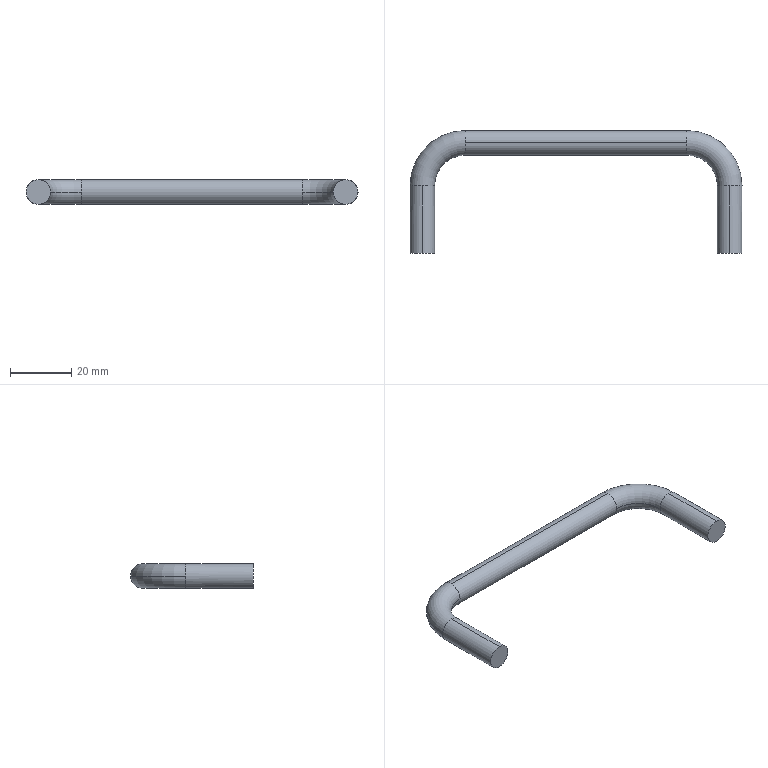Part | NX | features solid 2 | 1 solid | 12 faces | box 108 x 40 x 8 mm | volume 8042 mm3 | cylinder 6 | torus 4 | plane 2 | commonest cylinder face diameters 8 x6
STEP:
#1=CARTESIAN_POINT('',(1515.,-645.,1049.));
#2=VERTEX_POINT('',#1);
#3=CARTESIAN_POINT('',(1515.,-623.,1049.));
#4=VERTEX_POINT('',#3);
#5=CARTESIAN_POINT('',(1515.,-623.,1049.));
#6=DIRECTION('',(0.,1.,0.));
#7=VECTOR('',#6,1000.);
#8=LINE('',#5,#7);
#9=EDGE_CURVE('',#2,#4,#8,.T.);
#10=ORIENTED_EDGE('',*,*,#9,.F.);
#11=CARTESIAN_POINT('',(1515.,-645.,1041.));
#12=VERTEX_POINT('',#11);
#13=CARTESIAN_POINT('',(1515.,-645.,1045.));
#14=DIRECTION('',(0.,-1.,0.));
#15=DIRECTION('',(-1.,0.,0.));
#16=AXIS2_PLACEMENT_3D('',#13,#14,#15);
#17=CIRCLE('',#16,4.);
#18=EDGE_CURVE('',#12,#2,#17,.T.);
#19=ORIENTED_EDGE('',*,*,#18,.F.);
#20=CARTESIAN_POINT('',(1515.,-623.,1041.));
#21=VERTEX_POINT('',#20);
#22=CARTESIAN_POINT('',(1515.,-623.,1041.));
#23=DIRECTION('',(0.,1.,0.));
#24=VECTOR('',#23,1000.);
#25=LINE('',#22,#24);
#26=EDGE_CURVE('',#21,#12,#25,.F.);
#27=ORIENTED_EDGE('',*,*,#26,.F.);
#28=CARTESIAN_POINT('',(1519.,-623.,1045.));
#29=VERTEX_POINT('',#28);
#30=CARTESIAN_POINT('',(1515.,-623.,1045.));
#31=DIRECTION('',(0.,-1.,0.));
#32=DIRECTION('',(0.,0.,1.));
#33=AXIS2_PLACEMENT_3D('',#30,#31,#32);
#34=CIRCLE('',#33,4.);
#35=EDGE_CURVE('',#21,#29,#34,.T.);
#36=ORIENTED_EDGE('',*,*,#35,.T.);
#37=CARTESIAN_POINT('',(1515.,-623.,1045.));
#38=DIRECTION('',(0.,-1.,0.));
#39=DIRECTION('',(0.,0.,1.));
#40=AXIS2_PLACEMENT_3D('',#37,#38,#39);
#41=CIRCLE('',#40,4.);
#42=EDGE_CURVE('',#29,#4,#41,.T.);
#43=ORIENTED_EDGE('',*,*,#42,.T.);
#44=EDGE_LOOP('',(#10,#19,#27,#36,#43));
#45=FACE_BOUND('',#44,.T.);
#46=CARTESIAN_POINT('',(1515.,-623.,1045.));
#47=DIRECTION('',(0.,1.,0.));
#48=DIRECTION('',(0.,0.,-1.));
#49=AXIS2_PLACEMENT_3D('',#46,#47,#48);
#50=CYLINDRICAL_SURFACE('',#49,4.);
#51=ADVANCED_FACE('',(#45),#50,.T.);
#52=CARTESIAN_POINT('',(1529.,-605.,1045.));
#53=VERTEX_POINT('',#52);
#54=CARTESIAN_POINT('',(1511.,-623.,1045.));
#55=VERTEX_POINT('',#54);
#56=CARTESIAN_POINT('',(1529.,-623.,1045.));
#57=DIRECTION('',(0.,0.,1.));
#58=DIRECTION('',(1.,0.,0.));
#59=AXIS2_PLACEMENT_3D('',#56,#57,#58);
#60=CIRCLE('',#59,18.);
#61=EDGE_CURVE('',#53,#55,#60,.T.);
#62=ORIENTED_EDGE('',*,*,#61,.F.);
#63=CARTESIAN_POINT('',(1529.,-609.,1041.));
#64=VERTEX_POINT('',#63);
#65=CARTESIAN_POINT('',(1529.,-609.,1045.));
#66=DIRECTION('',(-1.,0.,0.));
#67=DIRECTION('',(0.,1.,0.));
#68=AXIS2_PLACEMENT_3D('',#65,#66,#67);
#69=CIRCLE('',#68,4.);
#70=EDGE_CURVE('',#53,#64,#69,.T.);
#71=ORIENTED_EDGE('',*,*,#70,.T.);
#72=CARTESIAN_POINT('',(1529.,-613.,1045.));
#73=VERTEX_POINT('',#72);
#74=CARTESIAN_POINT('',(1529.,-609.,1045.));
#75=DIRECTION('',(-1.,0.,0.));
#76=DIRECTION('',(0.,1.,0.));
#77=AXIS2_PLACEMENT_3D('',#74,#75,#76);
#78=CIRCLE('',#77,4.);
#79=EDGE_CURVE('',#64,#73,#78,.T.);
#80=ORIENTED_EDGE('',*,*,#79,.T.);
#81=CARTESIAN_POINT('',(1529.,-623.,1045.));
#82=DIRECTION('',(0.,0.,1.));
#83=DIRECTION('',(1.,0.,0.));
#84=AXIS2_PLACEMENT_3D('',#81,#82,#83);
#85=CIRCLE('',#84,10.);
#86=EDGE_CURVE('',#29,#73,#85,.F.);
#87=ORIENTED_EDGE('',*,*,#86,.F.);
#88=ORIENTED_EDGE('',*,*,#35,.F.);
#89=CARTESIAN_POINT('',(1515.,-623.,1045.));
#90=DIRECTION('',(0.,-1.,0.));
#91=DIRECTION('',(0.,0.,1.));
#92=AXIS2_PLACEMENT_3D('',#89,#90,#91);
#93=CIRCLE('',#92,4.);
#94=EDGE_CURVE('',#55,#21,#93,.T.);
#95=ORIENTED_EDGE('',*,*,#94,.F.);
#96=EDGE_LOOP('',(#62,#71,#80,#87,#88,#95));
#97=FACE_BOUND('',#96,.T.);
#98=CARTESIAN_POINT('',(1529.,-623.,1045.));
#99=DIRECTION('',(0.,0.,1.));
#100=DIRECTION('',(1.,0.,0.));
#101=AXIS2_PLACEMENT_3D('',#98,#99,#100);
#102=TOROIDAL_SURFACE('',#101,14.,4.);
#103=ADVANCED_FACE('',(#97),#102,.T.);
#104=CARTESIAN_POINT('',(1529.,-609.,1049.));
#105=VERTEX_POINT('',#104);
#106=CARTESIAN_POINT('',(1601.,-609.,1049.));
#107=VERTEX_POINT('',#106);
#108=CARTESIAN_POINT('',(1601.,-609.,1049.));
#109=DIRECTION('',(1.,0.,0.));
#110=VECTOR('',#109,1000.);
#111=LINE('',#108,#110);
#112=EDGE_CURVE('',#105,#107,#111,.T.);
#113=ORIENTED_EDGE('',*,*,#112,.F.);
#114=CARTESIAN_POINT('',(1529.,-609.,1045.));
#115=DIRECTION('',(-1.,0.,0.));
#116=DIRECTION('',(0.,1.,0.));
#117=AXIS2_PLACEMENT_3D('',#114,#115,#116);
#118=CIRCLE('',#117,4.);
#119=EDGE_CURVE('',#73,#105,#118,.T.);
#120=ORIENTED_EDGE('',*,*,#119,.F.);
#121=ORIENTED_EDGE('',*,*,#79,.F.);
#122=CARTESIAN_POINT('',(1601.,-609.,1041.));
#123=VERTEX_POINT('',#122);
#124=CARTESIAN_POINT('',(1601.,-609.,1041.));
#125=DIRECTION('',(1.,0.,0.));
#126=VECTOR('',#125,1000.);
#127=LINE('',#124,#126);
#128=EDGE_CURVE('',#123,#64,#127,.F.);
#129=ORIENTED_EDGE('',*,*,#128,.F.);
#130=CARTESIAN_POINT('',(1601.,-613.,1045.));
#131=VERTEX_POINT('',#130);
#132=CARTESIAN_POINT('',(1601.,-609.,1045.));
#133=DIRECTION('',(-1.,0.,0.));
#134=DIRECTION('',(0.,1.,0.));
#135=AXIS2_PLACEMENT_3D('',#132,#133,#134);
#136=CIRCLE('',#135,4.);
#137=EDGE_CURVE('',#123,#131,#136,.T.);
#138=ORIENTED_EDGE('',*,*,#137,.T.);
#139=CARTESIAN_POINT('',(1601.,-609.,1045.));
#140=DIRECTION('',(-1.,0.,0.));
#141=DIRECTION('',(0.,1.,0.));
#142=AXIS2_PLACEMENT_3D('',#139,#140,#141);
#143=CIRCLE('',#142,4.);
#144=EDGE_CURVE('',#131,#107,#143,.T.);
#145=ORIENTED_EDGE('',*,*,#144,.T.);
#146=EDGE_LOOP('',(#113,#120,#121,#129,#138,#145));
#147=FACE_BOUND('',#146,.T.);
#148=CARTESIAN_POINT('',(1601.,-609.,1045.));
#149=DIRECTION('',(1.,0.,0.));
#150=DIRECTION('',(0.,0.,-1.));
#151=AXIS2_PLACEMENT_3D('',#148,#149,#150);
#152=CYLINDRICAL_SURFACE('',#151,4.);
#153=ADVANCED_FACE('',(#147),#152,.T.);
#154=CARTESIAN_POINT('',(1619.,-623.,1045.));
#155=VERTEX_POINT('',#154);
#156=CARTESIAN_POINT('',(1601.,-605.,1045.));
#157=VERTEX_POINT('',#156);
#158=CARTESIAN_POINT('',(1601.,-623.,1045.));
#159=DIRECTION('',(0.,0.,1.));
#160=DIRECTION('',(1.,0.,0.));
#161=AXIS2_PLACEMENT_3D('',#158,#159,#160);
#162=CIRCLE('',#161,18.);
#163=EDGE_CURVE('',#155,#157,#162,.T.);
#164=ORIENTED_EDGE('',*,*,#163,.F.);
#165=CARTESIAN_POINT('',(1615.,-623.,1041.));
#166=VERTEX_POINT('',#165);
#167=CARTESIAN_POINT('',(1615.,-623.,1045.));
#168=DIRECTION('',(0.,1.,0.));
#169=DIRECTION('',(0.,0.,-1.));
#170=AXIS2_PLACEMENT_3D('',#167,#168,#169);
#171=CIRCLE('',#170,4.);
#172=EDGE_CURVE('',#155,#166,#171,.T.);
#173=ORIENTED_EDGE('',*,*,#172,.T.);
#174=CARTESIAN_POINT('',(1611.,-623.,1045.));
#175=VERTEX_POINT('',#174);
#176=CARTESIAN_POINT('',(1615.,-623.,1045.));
#177=DIRECTION('',(0.,1.,0.));
#178=DIRECTION('',(0.,0.,-1.));
#179=AXIS2_PLACEMENT_3D('',#176,#177,#178);
#180=CIRCLE('',#179,4.);
#181=EDGE_CURVE('',#166,#175,#180,.T.);
#182=ORIENTED_EDGE('',*,*,#181,.T.);
#183=CARTESIAN_POINT('',(1601.,-623.,1045.));
#184=DIRECTION('',(0.,0.,1.));
#185=DIRECTION('',(1.,0.,0.));
#186=AXIS2_PLACEMENT_3D('',#183,#184,#185);
#187=CIRCLE('',#186,10.);
#188=EDGE_CURVE('',#131,#175,#187,.F.);
#189=ORIENTED_EDGE('',*,*,#188,.F.);
#190=ORIENTED_EDGE('',*,*,#137,.F.);
#191=CARTESIAN_POINT('',(1601.,-609.,1045.));
#192=DIRECTION('',(-1.,0.,0.));
#193=DIRECTION('',(0.,1.,0.));
#194=AXIS2_PLACEMENT_3D('',#191,#192,#193);
#195=CIRCLE('',#194,4.);
#196=EDGE_CURVE('',#157,#123,#195,.T.);
#197=ORIENTED_EDGE('',*,*,#196,.F.);
#198=EDGE_LOOP('',(#164,#173,#182,#189,#190,#197));
#199=FACE_BOUND('',#198,.T.);
#200=CARTESIAN_POINT('',(1601.,-623.,1045.));
#201=DIRECTION('',(0.,0.,1.));
#202=DIRECTION('',(1.,0.,0.));
#203=AXIS2_PLACEMENT_3D('',#200,#201,#202);
#204=TOROIDAL_SURFACE('',#203,14.,4.);
#205=ADVANCED_FACE('',(#199),#204,.T.);
#206=CARTESIAN_POINT('',(1615.,-645.,1041.));
#207=VERTEX_POINT('',#206);
#208=CARTESIAN_POINT('',(1615.,-645.,1041.));
#209=DIRECTION('',(0.,-1.,0.));
#210=VECTOR('',#209,1000.);
#211=LINE('',#208,#210);
#212=EDGE_CURVE('',#166,#207,#211,.T.);
#213=ORIENTED_EDGE('',*,*,#212,.F.);
#214=ORIENTED_EDGE('',*,*,#172,.F.);
#215=CARTESIAN_POINT('',(1615.,-623.,1049.));
#216=VERTEX_POINT('',#215);
#217=CARTESIAN_POINT('',(1615.,-623.,1045.));
#218=DIRECTION('',(0.,1.,0.));
#219=DIRECTION('',(0.,0.,-1.));
#220=AXIS2_PLACEMENT_3D('',#217,#218,#219);
#221=CIRCLE('',#220,4.);
#222=EDGE_CURVE('',#216,#155,#221,.T.);
#223=ORIENTED_EDGE('',*,*,#222,.F.);
#224=CARTESIAN_POINT('',(1615.,-645.,1049.));
#225=VERTEX_POINT('',#224);
#226=CARTESIAN_POINT('',(1615.,-645.,1049.));
#227=DIRECTION('',(0.,-1.,0.));
#228=VECTOR('',#227,1000.);
#229=LINE('',#226,#228);
#230=EDGE_CURVE('',#225,#216,#229,.F.);
#231=ORIENTED_EDGE('',*,*,#230,.F.);
#232=CARTESIAN_POINT('',(1615.,-645.,1045.));
#233=DIRECTION('',(0.,-1.,0.));
#234=DIRECTION('',(-1.,0.,0.));
#235=AXIS2_PLACEMENT_3D('',#232,#233,#234);
#236=CIRCLE('',#235,4.);
#237=EDGE_CURVE('',#207,#225,#236,.T.);
#238=ORIENTED_EDGE('',*,*,#237,.F.);
#239=EDGE_LOOP('',(#213,#214,#223,#231,#238));
#240=FACE_BOUND('',#239,.T.);
#241=CARTESIAN_POINT('',(1615.,-645.,1045.));
#242=DIRECTION('',(0.,-1.,0.));
#243=DIRECTION('',(0.,0.,1.));
#244=AXIS2_PLACEMENT_3D('',#241,#242,#243);
#245=CYLINDRICAL_SURFACE('',#244,4.);
#246=ADVANCED_FACE('',(#240),#245,.T.);
#247=ORIENTED_EDGE('',*,*,#18,.T.);
#248=CARTESIAN_POINT('',(1515.,-645.,1045.));
#249=DIRECTION('',(0.,-1.,0.));
#250=DIRECTION('',(-1.,0.,0.));
#251=AXIS2_PLACEMENT_3D('',#248,#249,#250);
#252=CIRCLE('',#251,4.);
#253=EDGE_CURVE('',#2,#12,#252,.T.);
#254=ORIENTED_EDGE('',*,*,#253,.T.);
#255=EDGE_LOOP('',(#247,#254));
#256=FACE_BOUND('',#255,.T.);
#257=CARTESIAN_POINT('',(1511.,-645.,1041.));
#258=DIRECTION('',(0.,-1.,0.));
#259=DIRECTION('',(-1.,0.,0.));
#260=AXIS2_PLACEMENT_3D('',#257,#258,#259);
#261=PLANE('',#260);
#262=ADVANCED_FACE('',(#256),#261,.T.);
#263=CARTESIAN_POINT('',(1615.,-645.,1045.));
#264=DIRECTION('',(0.,-1.,0.));
#265=DIRECTION('',(-1.,0.,0.));
#266=AXIS2_PLACEMENT_3D('',#263,#264,#265);
#267=CIRCLE('',#266,4.);
#268=EDGE_CURVE('',#225,#207,#267,.T.);
#269=ORIENTED_EDGE('',*,*,#268,.T.);
#270=ORIENTED_EDGE('',*,*,#237,.T.);
#271=EDGE_LOOP('',(#269,#270));
#272=FACE_BOUND('',#271,.T.);
#273=CARTESIAN_POINT('',(1611.,-645.,1041.));
#274=DIRECTION('',(0.,-1.,0.));
#275=DIRECTION('',(-1.,0.,0.));
#276=AXIS2_PLACEMENT_3D('',#273,#274,#275);
#277=PLANE('',#276);
#278=ADVANCED_FACE('',(#272),#277,.T.);
#279=ORIENTED_EDGE('',*,*,#181,.F.);
#280=ORIENTED_EDGE('',*,*,#212,.T.);
#281=ORIENTED_EDGE('',*,*,#268,.F.);
#282=ORIENTED_EDGE('',*,*,#230,.T.);
#283=CARTESIAN_POINT('',(1615.,-623.,1045.));
#284=DIRECTION('',(0.,1.,0.));
#285=DIRECTION('',(0.,0.,-1.));
#286=AXIS2_PLACEMENT_3D('',#283,#284,#285);
#287=CIRCLE('',#286,4.);
#288=EDGE_CURVE('',#175,#216,#287,.T.);
#289=ORIENTED_EDGE('',*,*,#288,.F.);
#290=EDGE_LOOP('',(#279,#280,#281,#282,#289));
#291=FACE_BOUND('',#290,.T.);
#292=CARTESIAN_POINT('',(1615.,-645.,1045.));
#293=DIRECTION('',(0.,-1.,0.));
#294=DIRECTION('',(0.,0.,1.));
#295=AXIS2_PLACEMENT_3D('',#292,#293,#294);
#296=CYLINDRICAL_SURFACE('',#295,4.);
#297=ADVANCED_FACE('',(#291),#296,.T.);
#298=CARTESIAN_POINT('',(1529.,-609.,1045.));
#299=DIRECTION('',(-1.,0.,0.));
#300=DIRECTION('',(0.,1.,0.));
#301=AXIS2_PLACEMENT_3D('',#298,#299,#300);
#302=CIRCLE('',#301,4.);
#303=EDGE_CURVE('',#105,#53,#302,.T.);
#304=ORIENTED_EDGE('',*,*,#303,.F.);
#305=ORIENTED_EDGE('',*,*,#112,.T.);
#306=CARTESIAN_POINT('',(1601.,-609.,1045.));
#307=DIRECTION('',(-1.,0.,0.));
#308=DIRECTION('',(0.,1.,0.));
#309=AXIS2_PLACEMENT_3D('',#306,#307,#308);
#310=CIRCLE('',#309,4.);
#311=EDGE_CURVE('',#107,#157,#310,.T.);
#312=ORIENTED_EDGE('',*,*,#311,.T.);
#313=ORIENTED_EDGE('',*,*,#196,.T.);
#314=ORIENTED_EDGE('',*,*,#128,.T.);
#315=ORIENTED_EDGE('',*,*,#70,.F.);
#316=EDGE_LOOP('',(#304,#305,#312,#313,#314,#315));
#317=FACE_BOUND('',#316,.T.);
#318=CARTESIAN_POINT('',(1601.,-609.,1045.));
#319=DIRECTION('',(1.,0.,0.));
#320=DIRECTION('',(0.,0.,-1.));
#321=AXIS2_PLACEMENT_3D('',#318,#319,#320);
#322=CYLINDRICAL_SURFACE('',#321,4.);
#323=ADVANCED_FACE('',(#317),#322,.T.);
#324=ORIENTED_EDGE('',*,*,#253,.F.);
#325=ORIENTED_EDGE('',*,*,#9,.T.);
#326=CARTESIAN_POINT('',(1515.,-623.,1045.));
#327=DIRECTION('',(0.,-1.,0.));
#328=DIRECTION('',(0.,0.,1.));
#329=AXIS2_PLACEMENT_3D('',#326,#327,#328);
#330=CIRCLE('',#329,4.);
#331=EDGE_CURVE('',#4,#55,#330,.T.);
#332=ORIENTED_EDGE('',*,*,#331,.T.);
#333=ORIENTED_EDGE('',*,*,#94,.T.);
#334=ORIENTED_EDGE('',*,*,#26,.T.);
#335=EDGE_LOOP('',(#324,#325,#332,#333,#334));
#336=FACE_BOUND('',#335,.T.);
#337=CARTESIAN_POINT('',(1515.,-623.,1045.));
#338=DIRECTION('',(0.,1.,0.));
#339=DIRECTION('',(0.,0.,-1.));
#340=AXIS2_PLACEMENT_3D('',#337,#338,#339);
#341=CYLINDRICAL_SURFACE('',#340,4.);
#342=ADVANCED_FACE('',(#336),#341,.T.);
#343=ORIENTED_EDGE('',*,*,#222,.T.);
#344=ORIENTED_EDGE('',*,*,#163,.T.);
#345=ORIENTED_EDGE('',*,*,#311,.F.);
#346=ORIENTED_EDGE('',*,*,#144,.F.);
#347=ORIENTED_EDGE('',*,*,#188,.T.);
#348=ORIENTED_EDGE('',*,*,#288,.T.);
#349=EDGE_LOOP('',(#343,#344,#345,#346,#347,#348));
#350=FACE_BOUND('',#349,.T.);
#351=CARTESIAN_POINT('',(1601.,-623.,1045.));
#352=DIRECTION('',(0.,0.,1.));
#353=DIRECTION('',(1.,0.,0.));
#354=AXIS2_PLACEMENT_3D('',#351,#352,#353);
#355=TOROIDAL_SURFACE('',#354,14.,4.);
#356=ADVANCED_FACE('',(#350),#355,.T.);
#357=ORIENTED_EDGE('',*,*,#303,.T.);
#358=ORIENTED_EDGE('',*,*,#61,.T.);
#359=ORIENTED_EDGE('',*,*,#331,.F.);
#360=ORIENTED_EDGE('',*,*,#42,.F.);
#361=ORIENTED_EDGE('',*,*,#86,.T.);
#362=ORIENTED_EDGE('',*,*,#119,.T.);
#363=EDGE_LOOP('',(#357,#358,#359,#360,#361,#362));
#364=FACE_BOUND('',#363,.T.);
#365=CARTESIAN_POINT('',(1529.,-623.,1045.));
#366=DIRECTION('',(0.,0.,1.));
#367=DIRECTION('',(1.,0.,0.));
#368=AXIS2_PLACEMENT_3D('',#365,#366,#367);
#369=TOROIDAL_SURFACE('',#368,14.,4.);
#370=ADVANCED_FACE('',(#364),#369,.T.);
#371=CLOSED_SHELL('',(#51,#103,#153,#205,#246,#262,#278,#297,#323,#342,#356,#370));
#372=MANIFOLD_SOLID_BREP('',#371);
#373=(LENGTH_UNIT()NAMED_UNIT(*)SI_UNIT(.MILLI.,.METRE.));
#374=UNCERTAINTY_MEASURE_WITH_UNIT(LENGTH_MEASURE(0.00001),#373,'','');
#375=(NAMED_UNIT(*)PLANE_ANGLE_UNIT()SI_UNIT($,.RADIAN.));
#376=(NAMED_UNIT(*)SI_UNIT($,.STERADIAN.)SOLID_ANGLE_UNIT());
#377=(GEOMETRIC_REPRESENTATION_CONTEXT(3)GLOBAL_UNCERTAINTY_ASSIGNED_CONTEXT((#374))GLOBAL_UNIT_ASSIGNED_CONTEXT((#373,#375,#376))REPRESENTATION_CONTEXT('',''));
#378=ADVANCED_BREP_SHAPE_REPRESENTATION('',(#372),#377);